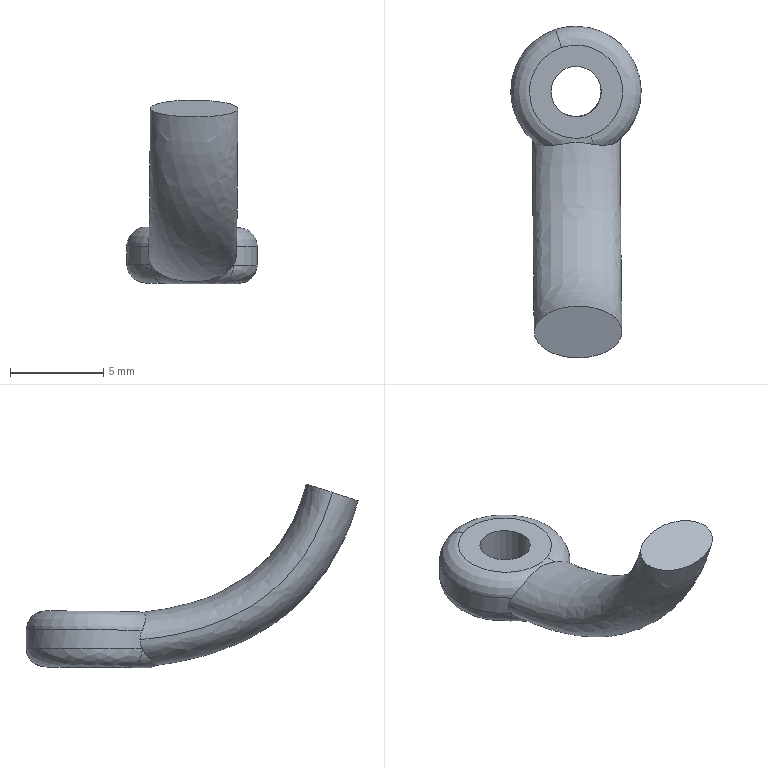Part | STEP file | Wytnij-wyci_gni_cie10 | 1 solid | 12 faces | box 7.005 x 17.81 x 9.853 mm | volume 233.546 mm3 | spline 6 | plane 3 | cylinder 3 | commonest cylinder face diameters 7 x2 2.7 x1